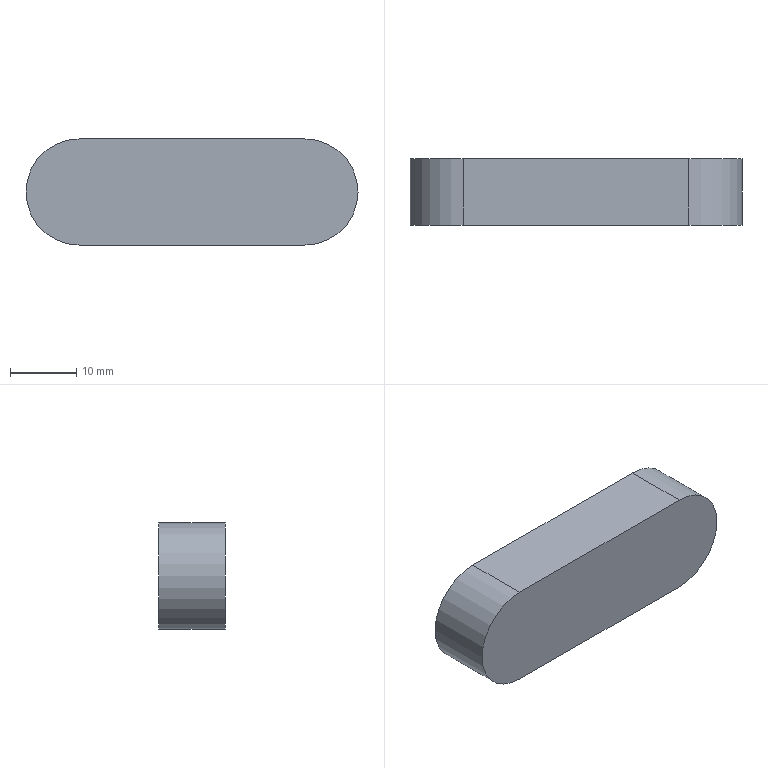Part | SolidWorks | features Extrusion 1 | 1 solid | 6 faces | box 50 x 10 x 16 mm | volume 7451 mm3 | plane 4 | cylinder 2 | commonest cylinder face diameters 16 x2
STEP:
#1=CARTESIAN_POINT('',(0.,0.,-8.));
#2=VERTEX_POINT('',#1);
#3=CARTESIAN_POINT('',(0.,0.,8.));
#4=VERTEX_POINT('',#3);
#5=CARTESIAN_POINT('',(0.,0.,0.));
#6=DIRECTION('',(0.,1.,0.));
#7=DIRECTION('',(0.,0.,1.));
#8=AXIS2_PLACEMENT_3D('',#5,#6,#7);
#9=CIRCLE('',#8,8.);
#10=EDGE_CURVE('',#2,#4,#9,.T.);
#11=ORIENTED_EDGE('',*,*,#10,.T.);
#12=CARTESIAN_POINT('',(0.,10.,8.));
#13=VERTEX_POINT('',#12);
#14=CARTESIAN_POINT('',(0.,10.,8.));
#15=DIRECTION('',(0.,-1.,0.));
#16=VECTOR('',#15,1000.);
#17=LINE('',#14,#16);
#18=EDGE_CURVE('',#13,#4,#17,.T.);
#19=ORIENTED_EDGE('',*,*,#18,.F.);
#20=CARTESIAN_POINT('',(0.,10.,-8.));
#21=VERTEX_POINT('',#20);
#22=CARTESIAN_POINT('',(0.,10.,0.));
#23=DIRECTION('',(0.,1.,0.));
#24=DIRECTION('',(0.,0.,1.));
#25=AXIS2_PLACEMENT_3D('',#22,#23,#24);
#26=CIRCLE('',#25,8.);
#27=EDGE_CURVE('',#21,#13,#26,.T.);
#28=ORIENTED_EDGE('',*,*,#27,.F.);
#29=CARTESIAN_POINT('',(0.,10.,-8.));
#30=DIRECTION('',(0.,-1.,0.));
#31=VECTOR('',#30,1000.);
#32=LINE('',#29,#31);
#33=EDGE_CURVE('',#21,#2,#32,.T.);
#34=ORIENTED_EDGE('',*,*,#33,.T.);
#35=EDGE_LOOP('',(#11,#19,#28,#34));
#36=FACE_OUTER_BOUND('',#35,.T.);
#37=CARTESIAN_POINT('',(0.,10.,0.));
#38=DIRECTION('',(0.,-1.,0.));
#39=DIRECTION('',(0.,0.,-1.));
#40=AXIS2_PLACEMENT_3D('',#37,#38,#39);
#41=CYLINDRICAL_SURFACE('',#40,8.);
#42=ADVANCED_FACE('',(#36),#41,.T.);
#43=CARTESIAN_POINT('',(34.,0.,8.));
#44=VERTEX_POINT('',#43);
#45=CARTESIAN_POINT('',(0.,0.,8.));
#46=DIRECTION('',(1.,0.,0.));
#47=VECTOR('',#46,1000.);
#48=LINE('',#45,#47);
#49=EDGE_CURVE('',#4,#44,#48,.T.);
#50=ORIENTED_EDGE('',*,*,#49,.T.);
#51=CARTESIAN_POINT('',(34.,10.,8.));
#52=VERTEX_POINT('',#51);
#53=CARTESIAN_POINT('',(34.,10.,8.));
#54=DIRECTION('',(0.,-1.,0.));
#55=VECTOR('',#54,1000.);
#56=LINE('',#53,#55);
#57=EDGE_CURVE('',#52,#44,#56,.T.);
#58=ORIENTED_EDGE('',*,*,#57,.F.);
#59=CARTESIAN_POINT('',(0.,10.,8.));
#60=DIRECTION('',(1.,0.,0.));
#61=VECTOR('',#60,1000.);
#62=LINE('',#59,#61);
#63=EDGE_CURVE('',#13,#52,#62,.T.);
#64=ORIENTED_EDGE('',*,*,#63,.F.);
#65=ORIENTED_EDGE('',*,*,#18,.T.);
#66=EDGE_LOOP('',(#50,#58,#64,#65));
#67=FACE_OUTER_BOUND('',#66,.T.);
#68=CARTESIAN_POINT('',(0.,10.,8.));
#69=DIRECTION('',(0.,0.,-1.));
#70=DIRECTION('',(-1.,0.,0.));
#71=AXIS2_PLACEMENT_3D('',#68,#69,#70);
#72=PLANE('',#71);
#73=ADVANCED_FACE('',(#67),#72,.F.);
#74=CARTESIAN_POINT('',(34.,0.,-8.));
#75=VERTEX_POINT('',#74);
#76=CARTESIAN_POINT('',(34.,0.,0.));
#77=DIRECTION('',(0.,1.,0.));
#78=DIRECTION('',(0.,0.,1.));
#79=AXIS2_PLACEMENT_3D('',#76,#77,#78);
#80=CIRCLE('',#79,8.);
#81=EDGE_CURVE('',#44,#75,#80,.T.);
#82=ORIENTED_EDGE('',*,*,#81,.T.);
#83=CARTESIAN_POINT('',(34.,10.,-8.));
#84=VERTEX_POINT('',#83);
#85=CARTESIAN_POINT('',(34.,10.,-8.));
#86=DIRECTION('',(0.,-1.,0.));
#87=VECTOR('',#86,1000.);
#88=LINE('',#85,#87);
#89=EDGE_CURVE('',#84,#75,#88,.T.);
#90=ORIENTED_EDGE('',*,*,#89,.F.);
#91=CARTESIAN_POINT('',(34.,10.,0.));
#92=DIRECTION('',(0.,1.,0.));
#93=DIRECTION('',(0.,0.,1.));
#94=AXIS2_PLACEMENT_3D('',#91,#92,#93);
#95=CIRCLE('',#94,8.);
#96=EDGE_CURVE('',#52,#84,#95,.T.);
#97=ORIENTED_EDGE('',*,*,#96,.F.);
#98=ORIENTED_EDGE('',*,*,#57,.T.);
#99=EDGE_LOOP('',(#82,#90,#97,#98));
#100=FACE_OUTER_BOUND('',#99,.T.);
#101=CARTESIAN_POINT('',(34.,10.,0.));
#102=DIRECTION('',(0.,-1.,0.));
#103=DIRECTION('',(0.,0.,-1.));
#104=AXIS2_PLACEMENT_3D('',#101,#102,#103);
#105=CYLINDRICAL_SURFACE('',#104,8.);
#106=ADVANCED_FACE('',(#100),#105,.T.);
#107=CARTESIAN_POINT('',(0.,0.,-8.));
#108=DIRECTION('',(-1.,0.,0.));
#109=VECTOR('',#108,1000.);
#110=LINE('',#107,#109);
#111=EDGE_CURVE('',#75,#2,#110,.T.);
#112=ORIENTED_EDGE('',*,*,#111,.T.);
#113=ORIENTED_EDGE('',*,*,#33,.F.);
#114=CARTESIAN_POINT('',(0.,10.,-8.));
#115=DIRECTION('',(-1.,0.,0.));
#116=VECTOR('',#115,1000.);
#117=LINE('',#114,#116);
#118=EDGE_CURVE('',#84,#21,#117,.T.);
#119=ORIENTED_EDGE('',*,*,#118,.F.);
#120=ORIENTED_EDGE('',*,*,#89,.T.);
#121=EDGE_LOOP('',(#112,#113,#119,#120));
#122=FACE_OUTER_BOUND('',#121,.T.);
#123=CARTESIAN_POINT('',(0.,10.,-8.));
#124=DIRECTION('',(0.,0.,1.));
#125=DIRECTION('',(1.,0.,0.));
#126=AXIS2_PLACEMENT_3D('',#123,#124,#125);
#127=PLANE('',#126);
#128=ADVANCED_FACE('',(#122),#127,.F.);
#129=ORIENTED_EDGE('',*,*,#27,.T.);
#130=ORIENTED_EDGE('',*,*,#63,.T.);
#131=ORIENTED_EDGE('',*,*,#96,.T.);
#132=ORIENTED_EDGE('',*,*,#118,.T.);
#133=EDGE_LOOP('',(#129,#130,#131,#132));
#134=FACE_OUTER_BOUND('',#133,.T.);
#135=CARTESIAN_POINT('',(0.,10.,0.));
#136=DIRECTION('',(0.,1.,0.));
#137=DIRECTION('',(0.,0.,1.));
#138=AXIS2_PLACEMENT_3D('',#135,#136,#137);
#139=PLANE('',#138);
#140=ADVANCED_FACE('',(#134),#139,.T.);
#141=ORIENTED_EDGE('',*,*,#10,.F.);
#142=ORIENTED_EDGE('',*,*,#111,.F.);
#143=ORIENTED_EDGE('',*,*,#81,.F.);
#144=ORIENTED_EDGE('',*,*,#49,.F.);
#145=EDGE_LOOP('',(#141,#142,#143,#144));
#146=FACE_OUTER_BOUND('',#145,.T.);
#147=CARTESIAN_POINT('',(0.,0.,0.));
#148=DIRECTION('',(0.,1.,0.));
#149=DIRECTION('',(0.,0.,1.));
#150=AXIS2_PLACEMENT_3D('',#147,#148,#149);
#151=PLANE('',#150);
#152=ADVANCED_FACE('',(#146),#151,.F.);
#153=CLOSED_SHELL('',(#42,#73,#106,#128,#140,#152));
#154=MANIFOLD_SOLID_BREP('',#153);
#155=CARTESIAN_POINT('',(0.,0.,0.));
#156=DIRECTION('',(0.,0.,1.));
#157=DIRECTION('',(1.,0.,0.));
#158=AXIS2_PLACEMENT_3D('',#155,#156,#157);
#159=(LENGTH_UNIT()NAMED_UNIT(*)SI_UNIT(.MILLI.,.METRE.));
#160=UNCERTAINTY_MEASURE_WITH_UNIT(LENGTH_MEASURE(0.00001),#159,'','');
#161=(NAMED_UNIT(*)PLANE_ANGLE_UNIT()SI_UNIT($,.RADIAN.));
#162=(NAMED_UNIT(*)SI_UNIT($,.STERADIAN.)SOLID_ANGLE_UNIT());
#163=(GEOMETRIC_REPRESENTATION_CONTEXT(3)GLOBAL_UNCERTAINTY_ASSIGNED_CONTEXT((#160))GLOBAL_UNIT_ASSIGNED_CONTEXT((#159,#161,#162))REPRESENTATION_CONTEXT('',''));
#164=ADVANCED_BREP_SHAPE_REPRESENTATION('',(#154,#158),#163);